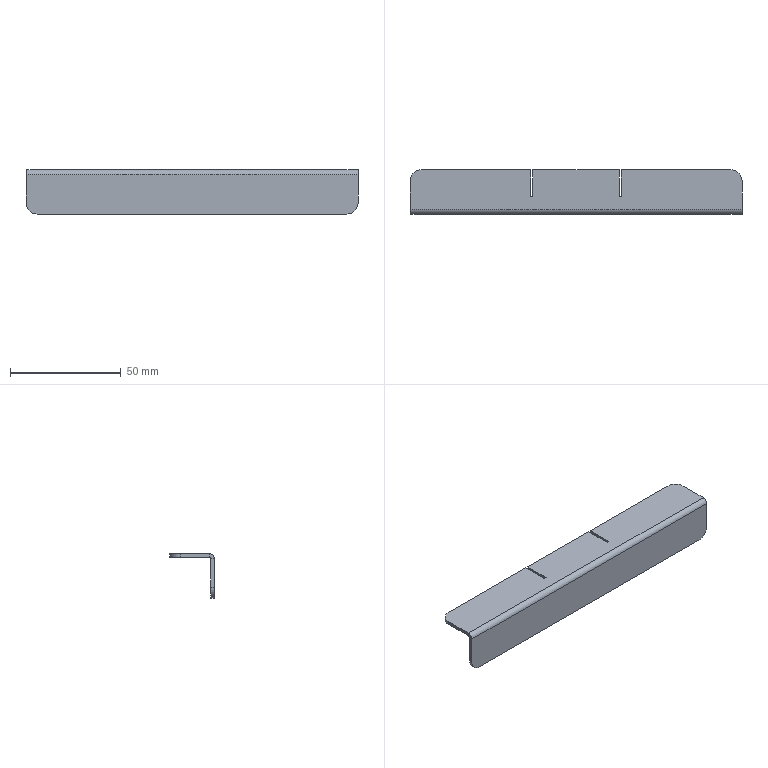Part | SolidWorks | features EdgeFlange 1, Fillet 1, FlatPattern 1, ICE 1, SMBaseFlange 1, SheetMetal 1 | 1 solid | 26 faces | box 150 x 20 x 20 mm | volume 8451 mm3 | plane 20 | cylinder 6 | commonest cylinder face diameters 10 x4 1.473 x1 4.473 x1
STEP:
#1=CARTESIAN_POINT('',(20.5,6.5,10.));
#2=VERTEX_POINT('',#1);
#3=CARTESIAN_POINT('',(19.5,6.5,10.));
#4=VERTEX_POINT('',#3);
#5=CARTESIAN_POINT('',(20.5,6.5,10.));
#6=DIRECTION('',(-1.,0.,0.));
#7=VECTOR('',#6,1000.);
#8=LINE('',#5,#7);
#9=EDGE_CURVE('',#2,#4,#8,.T.);
#10=ORIENTED_EDGE('',*,*,#9,.T.);
#11=CARTESIAN_POINT('',(19.5,18.5,10.));
#12=VERTEX_POINT('',#11);
#13=CARTESIAN_POINT('',(19.5,42.736,10.));
#14=DIRECTION('',(0.,1.,0.));
#15=VECTOR('',#14,1000.);
#16=LINE('',#13,#15);
#17=EDGE_CURVE('',#4,#12,#16,.T.);
#18=ORIENTED_EDGE('',*,*,#17,.T.);
#19=CARTESIAN_POINT('',(-19.5,18.5,10.));
#20=VERTEX_POINT('',#19);
#21=CARTESIAN_POINT('',(75.,18.5,10.));
#22=DIRECTION('',(1.,0.,0.));
#23=VECTOR('',#22,1000.);
#24=LINE('',#21,#23);
#25=EDGE_CURVE('',#20,#12,#24,.T.);
#26=ORIENTED_EDGE('',*,*,#25,.F.);
#27=CARTESIAN_POINT('',(-19.5,6.5,10.));
#28=VERTEX_POINT('',#27);
#29=CARTESIAN_POINT('',(-19.5,42.736,10.));
#30=DIRECTION('',(0.,-1.,0.));
#31=VECTOR('',#30,1000.);
#32=LINE('',#29,#31);
#33=EDGE_CURVE('',#20,#28,#32,.T.);
#34=ORIENTED_EDGE('',*,*,#33,.T.);
#35=CARTESIAN_POINT('',(-20.5,6.5,10.));
#36=VERTEX_POINT('',#35);
#37=CARTESIAN_POINT('',(-20.5,6.5,10.));
#38=DIRECTION('',(-1.,0.,0.));
#39=VECTOR('',#38,1000.);
#40=LINE('',#37,#39);
#41=EDGE_CURVE('',#28,#36,#40,.T.);
#42=ORIENTED_EDGE('',*,*,#41,.T.);
#43=CARTESIAN_POINT('',(-20.5,18.5,10.));
#44=VERTEX_POINT('',#43);
#45=CARTESIAN_POINT('',(-20.5,42.736,10.));
#46=DIRECTION('',(0.,1.,0.));
#47=VECTOR('',#46,1000.);
#48=LINE('',#45,#47);
#49=EDGE_CURVE('',#36,#44,#48,.T.);
#50=ORIENTED_EDGE('',*,*,#49,.T.);
#51=CARTESIAN_POINT('',(-70.,18.5,10.));
#52=VERTEX_POINT('',#51);
#53=CARTESIAN_POINT('',(75.,18.5,10.));
#54=DIRECTION('',(1.,0.,0.));
#55=VECTOR('',#54,1000.);
#56=LINE('',#53,#55);
#57=EDGE_CURVE('',#52,#44,#56,.T.);
#58=ORIENTED_EDGE('',*,*,#57,.F.);
#59=CARTESIAN_POINT('',(-75.,13.5,10.));
#60=VERTEX_POINT('',#59);
#61=CARTESIAN_POINT('',(-70.,13.5,10.));
#62=DIRECTION('',(0.,0.,1.));
#63=DIRECTION('',(0.,-1.,0.));
#64=AXIS2_PLACEMENT_3D('',#61,#62,#63);
#65=CIRCLE('',#64,5.);
#66=EDGE_CURVE('',#52,#60,#65,.T.);
#67=ORIENTED_EDGE('',*,*,#66,.T.);
#68=CARTESIAN_POINT('',(-75.,0.7366,10.));
#69=VERTEX_POINT('',#68);
#70=CARTESIAN_POINT('',(-75.,18.5,10.));
#71=DIRECTION('',(0.,1.,0.));
#72=VECTOR('',#71,1000.);
#73=LINE('',#70,#72);
#74=EDGE_CURVE('',#69,#60,#73,.T.);
#75=ORIENTED_EDGE('',*,*,#74,.F.);
#76=CARTESIAN_POINT('',(75.,0.7366,10.));
#77=VERTEX_POINT('',#76);
#78=CARTESIAN_POINT('',(0.,0.7366,10.));
#79=DIRECTION('',(1.,0.,0.));
#80=VECTOR('',#79,1000.);
#81=LINE('',#78,#80);
#82=EDGE_CURVE('',#69,#77,#81,.T.);
#83=ORIENTED_EDGE('',*,*,#82,.T.);
#84=CARTESIAN_POINT('',(75.,13.5,10.));
#85=VERTEX_POINT('',#84);
#86=CARTESIAN_POINT('',(75.,0.,10.));
#87=DIRECTION('',(0.,-1.,0.));
#88=VECTOR('',#87,1000.);
#89=LINE('',#86,#88);
#90=EDGE_CURVE('',#85,#77,#89,.T.);
#91=ORIENTED_EDGE('',*,*,#90,.F.);
#92=CARTESIAN_POINT('',(70.,18.5,10.));
#93=VERTEX_POINT('',#92);
#94=CARTESIAN_POINT('',(70.,13.5,10.));
#95=DIRECTION('',(0.,0.,1.));
#96=DIRECTION('',(0.,-1.,0.));
#97=AXIS2_PLACEMENT_3D('',#94,#95,#96);
#98=CIRCLE('',#97,5.);
#99=EDGE_CURVE('',#85,#93,#98,.T.);
#100=ORIENTED_EDGE('',*,*,#99,.T.);
#101=CARTESIAN_POINT('',(20.5,18.5,10.));
#102=VERTEX_POINT('',#101);
#103=CARTESIAN_POINT('',(75.,18.5,10.));
#104=DIRECTION('',(1.,0.,0.));
#105=VECTOR('',#104,1000.);
#106=LINE('',#103,#105);
#107=EDGE_CURVE('',#102,#93,#106,.T.);
#108=ORIENTED_EDGE('',*,*,#107,.F.);
#109=CARTESIAN_POINT('',(20.5,42.736,10.));
#110=DIRECTION('',(0.,-1.,0.));
#111=VECTOR('',#110,1000.);
#112=LINE('',#109,#111);
#113=EDGE_CURVE('',#102,#2,#112,.T.);
#114=ORIENTED_EDGE('',*,*,#113,.T.);
#115=EDGE_LOOP('',(#10,#18,#26,#34,#42,#50,#58,#67,#75,#83,#91,#100,#108,#114));
#116=FACE_OUTER_BOUND('',#115,.T.);
#117=CARTESIAN_POINT('',(0.,0.,10.));
#118=DIRECTION('',(0.,0.,1.));
#119=DIRECTION('',(0.,-1.,0.));
#120=AXIS2_PLACEMENT_3D('',#117,#118,#119);
#121=PLANE('',#120);
#122=ADVANCED_FACE('',(#116),#121,.T.);
#123=CARTESIAN_POINT('',(19.5,6.5,8.5));
#124=VERTEX_POINT('',#123);
#125=CARTESIAN_POINT('',(19.5,18.5,8.5));
#126=VERTEX_POINT('',#125);
#127=CARTESIAN_POINT('',(19.5,0.,8.5));
#128=DIRECTION('',(0.,1.,0.));
#129=VECTOR('',#128,1000.);
#130=LINE('',#127,#129);
#131=EDGE_CURVE('',#124,#126,#130,.T.);
#132=ORIENTED_EDGE('',*,*,#131,.F.);
#133=CARTESIAN_POINT('',(20.5,6.5,8.5));
#134=VERTEX_POINT('',#133);
#135=CARTESIAN_POINT('',(0.,6.5,8.5));
#136=DIRECTION('',(-1.,0.,0.));
#137=VECTOR('',#136,1000.);
#138=LINE('',#135,#137);
#139=EDGE_CURVE('',#134,#124,#138,.T.);
#140=ORIENTED_EDGE('',*,*,#139,.F.);
#141=CARTESIAN_POINT('',(20.5,18.5,8.5));
#142=VERTEX_POINT('',#141);
#143=CARTESIAN_POINT('',(20.5,0.,8.5));
#144=DIRECTION('',(0.,-1.,0.));
#145=VECTOR('',#144,1000.);
#146=LINE('',#143,#145);
#147=EDGE_CURVE('',#142,#134,#146,.T.);
#148=ORIENTED_EDGE('',*,*,#147,.F.);
#149=CARTESIAN_POINT('',(70.,18.5,8.5));
#150=VERTEX_POINT('',#149);
#151=CARTESIAN_POINT('',(0.,18.5,8.5));
#152=DIRECTION('',(1.,0.,0.));
#153=VECTOR('',#152,1000.);
#154=LINE('',#151,#153);
#155=EDGE_CURVE('',#142,#150,#154,.T.);
#156=ORIENTED_EDGE('',*,*,#155,.T.);
#157=CARTESIAN_POINT('',(75.,13.5,8.5));
#158=VERTEX_POINT('',#157);
#159=CARTESIAN_POINT('',(70.,13.5,8.5));
#160=DIRECTION('',(0.,0.,-1.));
#161=DIRECTION('',(0.,-1.,0.));
#162=AXIS2_PLACEMENT_3D('',#159,#160,#161);
#163=CIRCLE('',#162,5.);
#164=EDGE_CURVE('',#150,#158,#163,.T.);
#165=ORIENTED_EDGE('',*,*,#164,.T.);
#166=CARTESIAN_POINT('',(75.,0.7366,8.5));
#167=VERTEX_POINT('',#166);
#168=CARTESIAN_POINT('',(75.,0.,8.5));
#169=DIRECTION('',(0.,-1.,0.));
#170=VECTOR('',#169,1000.);
#171=LINE('',#168,#170);
#172=EDGE_CURVE('',#158,#167,#171,.T.);
#173=ORIENTED_EDGE('',*,*,#172,.T.);
#174=CARTESIAN_POINT('',(-75.,0.7366,8.5));
#175=VERTEX_POINT('',#174);
#176=CARTESIAN_POINT('',(-75.,0.7366,8.5));
#177=DIRECTION('',(1.,0.,0.));
#178=VECTOR('',#177,1000.);
#179=LINE('',#176,#178);
#180=EDGE_CURVE('',#175,#167,#179,.T.);
#181=ORIENTED_EDGE('',*,*,#180,.F.);
#182=CARTESIAN_POINT('',(-75.,13.5,8.5));
#183=VERTEX_POINT('',#182);
#184=CARTESIAN_POINT('',(-75.,0.,8.5));
#185=DIRECTION('',(0.,1.,0.));
#186=VECTOR('',#185,1000.);
#187=LINE('',#184,#186);
#188=EDGE_CURVE('',#175,#183,#187,.T.);
#189=ORIENTED_EDGE('',*,*,#188,.T.);
#190=CARTESIAN_POINT('',(-70.,18.5,8.5));
#191=VERTEX_POINT('',#190);
#192=CARTESIAN_POINT('',(-70.,13.5,8.5));
#193=DIRECTION('',(0.,0.,-1.));
#194=DIRECTION('',(0.,-1.,0.));
#195=AXIS2_PLACEMENT_3D('',#192,#193,#194);
#196=CIRCLE('',#195,5.);
#197=EDGE_CURVE('',#183,#191,#196,.T.);
#198=ORIENTED_EDGE('',*,*,#197,.T.);
#199=CARTESIAN_POINT('',(-20.5,18.5,8.5));
#200=VERTEX_POINT('',#199);
#201=CARTESIAN_POINT('',(0.,18.5,8.5));
#202=DIRECTION('',(1.,0.,0.));
#203=VECTOR('',#202,1000.);
#204=LINE('',#201,#203);
#205=EDGE_CURVE('',#191,#200,#204,.T.);
#206=ORIENTED_EDGE('',*,*,#205,.T.);
#207=CARTESIAN_POINT('',(-20.5,6.5,8.5));
#208=VERTEX_POINT('',#207);
#209=CARTESIAN_POINT('',(-20.5,0.,8.5));
#210=DIRECTION('',(0.,1.,0.));
#211=VECTOR('',#210,1000.);
#212=LINE('',#209,#211);
#213=EDGE_CURVE('',#208,#200,#212,.T.);
#214=ORIENTED_EDGE('',*,*,#213,.F.);
#215=CARTESIAN_POINT('',(-19.5,6.5,8.5));
#216=VERTEX_POINT('',#215);
#217=CARTESIAN_POINT('',(0.,6.5,8.5));
#218=DIRECTION('',(-1.,0.,0.));
#219=VECTOR('',#218,1000.);
#220=LINE('',#217,#219);
#221=EDGE_CURVE('',#216,#208,#220,.T.);
#222=ORIENTED_EDGE('',*,*,#221,.F.);
#223=CARTESIAN_POINT('',(-19.5,18.5,8.5));
#224=VERTEX_POINT('',#223);
#225=CARTESIAN_POINT('',(-19.5,0.,8.5));
#226=DIRECTION('',(0.,-1.,0.));
#227=VECTOR('',#226,1000.);
#228=LINE('',#225,#227);
#229=EDGE_CURVE('',#224,#216,#228,.T.);
#230=ORIENTED_EDGE('',*,*,#229,.F.);
#231=CARTESIAN_POINT('',(0.,18.5,8.5));
#232=DIRECTION('',(1.,0.,0.));
#233=VECTOR('',#232,1000.);
#234=LINE('',#231,#233);
#235=EDGE_CURVE('',#224,#126,#234,.T.);
#236=ORIENTED_EDGE('',*,*,#235,.T.);
#237=EDGE_LOOP('',(#132,#140,#148,#156,#165,#173,#181,#189,#198,#206,#214,#222,#230,#236));
#238=FACE_OUTER_BOUND('',#237,.T.);
#239=CARTESIAN_POINT('',(0.,0.,8.5));
#240=DIRECTION('',(0.,0.,1.));
#241=DIRECTION('',(0.,-1.,0.));
#242=AXIS2_PLACEMENT_3D('',#239,#240,#241);
#243=PLANE('',#242);
#244=ADVANCED_FACE('',(#238),#243,.F.);
#245=ORIENTED_EDGE('',*,*,#25,.T.);
#246=CARTESIAN_POINT('',(19.5,18.5,10.));
#247=DIRECTION('',(0.,0.,-1.));
#248=VECTOR('',#247,1000.);
#249=LINE('',#246,#248);
#250=EDGE_CURVE('',#12,#126,#249,.T.);
#251=ORIENTED_EDGE('',*,*,#250,.T.);
#252=ORIENTED_EDGE('',*,*,#235,.F.);
#253=CARTESIAN_POINT('',(-19.5,18.5,10.));
#254=DIRECTION('',(0.,0.,1.));
#255=VECTOR('',#254,1000.);
#256=LINE('',#253,#255);
#257=EDGE_CURVE('',#224,#20,#256,.T.);
#258=ORIENTED_EDGE('',*,*,#257,.T.);
#259=EDGE_LOOP('',(#245,#251,#252,#258));
#260=FACE_OUTER_BOUND('',#259,.T.);
#261=CARTESIAN_POINT('',(75.,18.5,10.));
#262=DIRECTION('',(0.,1.,0.));
#263=DIRECTION('',(0.,0.,1.));
#264=AXIS2_PLACEMENT_3D('',#261,#262,#263);
#265=PLANE('',#264);
#266=ADVANCED_FACE('',(#260),#265,.T.);
#267=ORIENTED_EDGE('',*,*,#155,.F.);
#268=CARTESIAN_POINT('',(20.5,18.5,10.));
#269=DIRECTION('',(0.,0.,1.));
#270=VECTOR('',#269,1000.);
#271=LINE('',#268,#270);
#272=EDGE_CURVE('',#142,#102,#271,.T.);
#273=ORIENTED_EDGE('',*,*,#272,.T.);
#274=ORIENTED_EDGE('',*,*,#107,.T.);
#275=CARTESIAN_POINT('',(70.,18.5,10.));
#276=DIRECTION('',(0.,0.,-1.));
#277=VECTOR('',#276,1000.);
#278=LINE('',#275,#277);
#279=EDGE_CURVE('',#93,#150,#278,.T.);
#280=ORIENTED_EDGE('',*,*,#279,.T.);
#281=EDGE_LOOP('',(#267,#273,#274,#280));
#282=FACE_OUTER_BOUND('',#281,.T.);
#283=CARTESIAN_POINT('',(75.,18.5,10.));
#284=DIRECTION('',(0.,1.,0.));
#285=DIRECTION('',(0.,0.,1.));
#286=AXIS2_PLACEMENT_3D('',#283,#284,#285);
#287=PLANE('',#286);
#288=ADVANCED_FACE('',(#282),#287,.T.);
#289=ORIENTED_EDGE('',*,*,#57,.T.);
#290=CARTESIAN_POINT('',(-20.5,18.5,10.));
#291=DIRECTION('',(0.,0.,-1.));
#292=VECTOR('',#291,1000.);
#293=LINE('',#290,#292);
#294=EDGE_CURVE('',#44,#200,#293,.T.);
#295=ORIENTED_EDGE('',*,*,#294,.T.);
#296=ORIENTED_EDGE('',*,*,#205,.F.);
#297=CARTESIAN_POINT('',(-70.,18.5,10.));
#298=DIRECTION('',(0.,0.,1.));
#299=VECTOR('',#298,1000.);
#300=LINE('',#297,#299);
#301=EDGE_CURVE('',#191,#52,#300,.T.);
#302=ORIENTED_EDGE('',*,*,#301,.T.);
#303=EDGE_LOOP('',(#289,#295,#296,#302));
#304=FACE_OUTER_BOUND('',#303,.T.);
#305=CARTESIAN_POINT('',(75.,18.5,10.));
#306=DIRECTION('',(0.,1.,0.));
#307=DIRECTION('',(0.,0.,1.));
#308=AXIS2_PLACEMENT_3D('',#305,#306,#307);
#309=PLANE('',#308);
#310=ADVANCED_FACE('',(#304),#309,.T.);
#311=CARTESIAN_POINT('',(75.,-1.5,7.763));
#312=VERTEX_POINT('',#311);
#313=CARTESIAN_POINT('',(75.,-1.5,-5.));
#314=VERTEX_POINT('',#313);
#315=CARTESIAN_POINT('',(75.,-1.5,-10.));
#316=DIRECTION('',(0.,0.,-1.));
#317=VECTOR('',#316,1000.);
#318=LINE('',#315,#317);
#319=EDGE_CURVE('',#312,#314,#318,.T.);
#320=ORIENTED_EDGE('',*,*,#319,.T.);
#321=CARTESIAN_POINT('',(75.,0.,-5.));
#322=VERTEX_POINT('',#321);
#323=CARTESIAN_POINT('',(75.,-1.5,-5.));
#324=DIRECTION('',(0.,1.,0.));
#325=VECTOR('',#324,1000.);
#326=LINE('',#323,#325);
#327=EDGE_CURVE('',#314,#322,#326,.T.);
#328=ORIENTED_EDGE('',*,*,#327,.T.);
#329=CARTESIAN_POINT('',(75.,0.,7.763));
#330=VERTEX_POINT('',#329);
#331=CARTESIAN_POINT('',(75.,0.,-10.));
#332=DIRECTION('',(0.,0.,-1.));
#333=VECTOR('',#332,1000.);
#334=LINE('',#331,#333);
#335=EDGE_CURVE('',#330,#322,#334,.T.);
#336=ORIENTED_EDGE('',*,*,#335,.F.);
#337=CARTESIAN_POINT('',(75.,0.,7.763));
#338=DIRECTION('',(0.,-1.,0.));
#339=VECTOR('',#338,1000.);
#340=LINE('',#337,#339);
#341=EDGE_CURVE('',#330,#312,#340,.T.);
#342=ORIENTED_EDGE('',*,*,#341,.T.);
#343=EDGE_LOOP('',(#320,#328,#336,#342));
#344=FACE_OUTER_BOUND('',#343,.T.);
#345=CARTESIAN_POINT('',(75.,-1.5,-10.));
#346=DIRECTION('',(1.,0.,0.));
#347=DIRECTION('',(0.,0.,-1.));
#348=AXIS2_PLACEMENT_3D('',#345,#346,#347);
#349=PLANE('',#348);
#350=ADVANCED_FACE('',(#344),#349,.T.);
#351=CARTESIAN_POINT('',(70.,-1.5,-10.));
#352=VERTEX_POINT('',#351);
#353=CARTESIAN_POINT('',(-70.,-1.5,-10.));
#354=VERTEX_POINT('',#353);
#355=CARTESIAN_POINT('',(-75.,-1.5,-10.));
#356=DIRECTION('',(-1.,0.,0.));
#357=VECTOR('',#356,1000.);
#358=LINE('',#355,#357);
#359=EDGE_CURVE('',#352,#354,#358,.T.);
#360=ORIENTED_EDGE('',*,*,#359,.F.);
#361=CARTESIAN_POINT('',(70.,-1.5,-5.));
#362=DIRECTION('',(0.,-1.,0.));
#363=DIRECTION('',(0.,0.,1.));
#364=AXIS2_PLACEMENT_3D('',#361,#362,#363);
#365=CIRCLE('',#364,5.);
#366=EDGE_CURVE('',#352,#314,#365,.T.);
#367=ORIENTED_EDGE('',*,*,#366,.T.);
#368=ORIENTED_EDGE('',*,*,#319,.F.);
#369=CARTESIAN_POINT('',(-75.,-1.5,7.763));
#370=VERTEX_POINT('',#369);
#371=CARTESIAN_POINT('',(75.,-1.5,7.763));
#372=DIRECTION('',(-1.,0.,0.));
#373=VECTOR('',#372,1000.);
#374=LINE('',#371,#373);
#375=EDGE_CURVE('',#312,#370,#374,.T.);
#376=ORIENTED_EDGE('',*,*,#375,.T.);
#377=CARTESIAN_POINT('',(-75.,-1.5,-5.));
#378=VERTEX_POINT('',#377);
#379=CARTESIAN_POINT('',(-75.,-1.5,-10.));
#380=DIRECTION('',(0.,0.,1.));
#381=VECTOR('',#380,1000.);
#382=LINE('',#379,#381);
#383=EDGE_CURVE('',#378,#370,#382,.T.);
#384=ORIENTED_EDGE('',*,*,#383,.F.);
#385=CARTESIAN_POINT('',(-70.,-1.5,-5.));
#386=DIRECTION('',(0.,-1.,0.));
#387=DIRECTION('',(0.,0.,1.));
#388=AXIS2_PLACEMENT_3D('',#385,#386,#387);
#389=CIRCLE('',#388,5.);
#390=EDGE_CURVE('',#378,#354,#389,.T.);
#391=ORIENTED_EDGE('',*,*,#390,.T.);
#392=EDGE_LOOP('',(#360,#367,#368,#376,#384,#391));
#393=FACE_OUTER_BOUND('',#392,.T.);
#394=CARTESIAN_POINT('',(0.,-1.5,0.));
#395=DIRECTION('',(0.,1.,0.));
#396=DIRECTION('',(0.,0.,1.));
#397=AXIS2_PLACEMENT_3D('',#394,#395,#396);
#398=PLANE('',#397);
#399=ADVANCED_FACE('',(#393),#398,.F.);
#400=ORIENTED_EDGE('',*,*,#335,.T.);
#401=CARTESIAN_POINT('',(70.,0.,-10.));
#402=VERTEX_POINT('',#401);
#403=CARTESIAN_POINT('',(70.,0.,-5.));
#404=DIRECTION('',(0.,1.,0.));
#405=DIRECTION('',(0.,0.,1.));
#406=AXIS2_PLACEMENT_3D('',#403,#404,#405);
#407=CIRCLE('',#406,5.);
#408=EDGE_CURVE('',#322,#402,#407,.T.);
#409=ORIENTED_EDGE('',*,*,#408,.T.);
#410=CARTESIAN_POINT('',(-70.,0.,-10.));
#411=VERTEX_POINT('',#410);
#412=CARTESIAN_POINT('',(-75.,0.,-10.));
#413=DIRECTION('',(-1.,0.,0.));
#414=VECTOR('',#413,1000.);
#415=LINE('',#412,#414);
#416=EDGE_CURVE('',#402,#411,#415,.T.);
#417=ORIENTED_EDGE('',*,*,#416,.T.);
#418=CARTESIAN_POINT('',(-75.,0.,-5.));
#419=VERTEX_POINT('',#418);
#420=CARTESIAN_POINT('',(-70.,0.,-5.));
#421=DIRECTION('',(0.,1.,0.));
#422=DIRECTION('',(0.,0.,1.));
#423=AXIS2_PLACEMENT_3D('',#420,#421,#422);
#424=CIRCLE('',#423,5.);
#425=EDGE_CURVE('',#411,#419,#424,.T.);
#426=ORIENTED_EDGE('',*,*,#425,.T.);
#427=CARTESIAN_POINT('',(-75.,0.,7.763));
#428=VERTEX_POINT('',#427);
#429=CARTESIAN_POINT('',(-75.,0.,-10.));
#430=DIRECTION('',(0.,0.,1.));
#431=VECTOR('',#430,1000.);
#432=LINE('',#429,#431);
#433=EDGE_CURVE('',#419,#428,#432,.T.);
#434=ORIENTED_EDGE('',*,*,#433,.T.);
#435=CARTESIAN_POINT('',(75.,0.,7.763));
#436=DIRECTION('',(-1.,0.,0.));
#437=VECTOR('',#436,1000.);
#438=LINE('',#435,#437);
#439=EDGE_CURVE('',#330,#428,#438,.T.);
#440=ORIENTED_EDGE('',*,*,#439,.F.);
#441=EDGE_LOOP('',(#400,#409,#417,#426,#434,#440));
#442=FACE_OUTER_BOUND('',#441,.T.);
#443=CARTESIAN_POINT('',(0.,0.,0.));
#444=DIRECTION('',(0.,1.,0.));
#445=DIRECTION('',(0.,0.,1.));
#446=AXIS2_PLACEMENT_3D('',#443,#444,#445);
#447=PLANE('',#446);
#448=ADVANCED_FACE('',(#442),#447,.T.);
#449=ORIENTED_EDGE('',*,*,#433,.F.);
#450=CARTESIAN_POINT('',(-75.,-1.5,-5.));
#451=DIRECTION('',(0.,-1.,0.));
#452=VECTOR('',#451,1000.);
#453=LINE('',#450,#452);
#454=EDGE_CURVE('',#419,#378,#453,.T.);
#455=ORIENTED_EDGE('',*,*,#454,.T.);
#456=ORIENTED_EDGE('',*,*,#383,.T.);
#457=CARTESIAN_POINT('',(-75.,0.,7.763));
#458=DIRECTION('',(0.,-1.,0.));
#459=VECTOR('',#458,1000.);
#460=LINE('',#457,#459);
#461=EDGE_CURVE('',#428,#370,#460,.T.);
#462=ORIENTED_EDGE('',*,*,#461,.F.);
#463=EDGE_LOOP('',(#449,#455,#456,#462));
#464=FACE_OUTER_BOUND('',#463,.T.);
#465=CARTESIAN_POINT('',(-75.,-1.5,-10.));
#466=DIRECTION('',(-1.,0.,0.));
#467=DIRECTION('',(0.,0.,1.));
#468=AXIS2_PLACEMENT_3D('',#465,#466,#467);
#469=PLANE('',#468);
#470=ADVANCED_FACE('',(#464),#469,.T.);
#471=ORIENTED_EDGE('',*,*,#416,.F.);
#472=CARTESIAN_POINT('',(70.,-1.5,-10.));
#473=DIRECTION('',(0.,-1.,0.));
#474=VECTOR('',#473,1000.);
#475=LINE('',#472,#474);
#476=EDGE_CURVE('',#402,#352,#475,.T.);
#477=ORIENTED_EDGE('',*,*,#476,.T.);
#478=ORIENTED_EDGE('',*,*,#359,.T.);
#479=CARTESIAN_POINT('',(-70.,-1.5,-10.));
#480=DIRECTION('',(0.,1.,0.));
#481=VECTOR('',#480,1000.);
#482=LINE('',#479,#481);
#483=EDGE_CURVE('',#354,#411,#482,.T.);
#484=ORIENTED_EDGE('',*,*,#483,.T.);
#485=EDGE_LOOP('',(#471,#477,#478,#484));
#486=FACE_OUTER_BOUND('',#485,.T.);
#487=CARTESIAN_POINT('',(-75.,-1.5,-10.));
#488=DIRECTION('',(0.,0.,-1.));
#489=DIRECTION('',(-1.,0.,0.));
#490=AXIS2_PLACEMENT_3D('',#487,#488,#489);
#491=PLANE('',#490);
#492=ADVANCED_FACE('',(#486),#491,.T.);
#493=CARTESIAN_POINT('',(-75.,0.7366,10.));
#494=DIRECTION('',(0.,0.,1.));
#495=VECTOR('',#494,1000.);
#496=LINE('',#493,#495);
#497=EDGE_CURVE('',#175,#69,#496,.T.);
#498=ORIENTED_EDGE('',*,*,#497,.F.);
#499=CARTESIAN_POINT('',(-75.,0.7366,7.763));
#500=DIRECTION('',(-1.,0.,0.));
#501=DIRECTION('',(0.,0.,-1.));
#502=AXIS2_PLACEMENT_3D('',#499,#500,#501);
#503=CIRCLE('',#502,0.7366);
#504=EDGE_CURVE('',#428,#175,#503,.T.);
#505=ORIENTED_EDGE('',*,*,#504,.F.);
#506=ORIENTED_EDGE('',*,*,#461,.T.);
#507=CARTESIAN_POINT('',(-75.,0.7366,7.763));
#508=DIRECTION('',(-1.,0.,0.));
#509=DIRECTION('',(0.,0.,-1.));
#510=AXIS2_PLACEMENT_3D('',#507,#508,#509);
#511=CIRCLE('',#510,2.237);
#512=EDGE_CURVE('',#370,#69,#511,.T.);
#513=ORIENTED_EDGE('',*,*,#512,.T.);
#514=EDGE_LOOP('',(#498,#505,#506,#513));
#515=FACE_OUTER_BOUND('',#514,.T.);
#516=CARTESIAN_POINT('',(-75.,0.7366,7.763));
#517=DIRECTION('',(-1.,0.,0.));
#518=DIRECTION('',(0.,0.,1.));
#519=AXIS2_PLACEMENT_3D('',#516,#517,#518);
#520=PLANE('',#519);
#521=ADVANCED_FACE('',(#515),#520,.T.);
#522=CARTESIAN_POINT('',(75.,0.7366,7.763));
#523=DIRECTION('',(1.,0.,0.));
#524=DIRECTION('',(0.,0.,-1.));
#525=AXIS2_PLACEMENT_3D('',#522,#523,#524);
#526=CIRCLE('',#525,0.7366);
#527=EDGE_CURVE('',#167,#330,#526,.T.);
#528=ORIENTED_EDGE('',*,*,#527,.F.);
#529=CARTESIAN_POINT('',(75.,0.7366,8.5));
#530=DIRECTION('',(0.,0.,1.));
#531=VECTOR('',#530,1000.);
#532=LINE('',#529,#531);
#533=EDGE_CURVE('',#167,#77,#532,.T.);
#534=ORIENTED_EDGE('',*,*,#533,.T.);
#535=CARTESIAN_POINT('',(75.,0.7366,7.763));
#536=DIRECTION('',(1.,0.,0.));
#537=DIRECTION('',(0.,0.,-1.));
#538=AXIS2_PLACEMENT_3D('',#535,#536,#537);
#539=CIRCLE('',#538,2.237);
#540=EDGE_CURVE('',#77,#312,#539,.T.);
#541=ORIENTED_EDGE('',*,*,#540,.T.);
#542=ORIENTED_EDGE('',*,*,#341,.F.);
#543=EDGE_LOOP('',(#528,#534,#541,#542));
#544=FACE_OUTER_BOUND('',#543,.T.);
#545=CARTESIAN_POINT('',(75.,0.7366,7.763));
#546=DIRECTION('',(-1.,0.,0.));
#547=DIRECTION('',(0.,0.,1.));
#548=AXIS2_PLACEMENT_3D('',#545,#546,#547);
#549=PLANE('',#548);
#550=ADVANCED_FACE('',(#544),#549,.F.);
#551=ORIENTED_EDGE('',*,*,#375,.F.);
#552=ORIENTED_EDGE('',*,*,#540,.F.);
#553=ORIENTED_EDGE('',*,*,#82,.F.);
#554=ORIENTED_EDGE('',*,*,#512,.F.);
#555=EDGE_LOOP('',(#551,#552,#553,#554));
#556=FACE_OUTER_BOUND('',#555,.T.);
#557=CARTESIAN_POINT('',(75.,0.7366,7.763));
#558=DIRECTION('',(1.,0.,0.));
#559=DIRECTION('',(0.,0.,1.));
#560=AXIS2_PLACEMENT_3D('',#557,#558,#559);
#561=CYLINDRICAL_SURFACE('',#560,2.237);
#562=ADVANCED_FACE('',(#556),#561,.T.);
#563=ORIENTED_EDGE('',*,*,#439,.T.);
#564=ORIENTED_EDGE('',*,*,#504,.T.);
#565=ORIENTED_EDGE('',*,*,#180,.T.);
#566=ORIENTED_EDGE('',*,*,#527,.T.);
#567=EDGE_LOOP('',(#563,#564,#565,#566));
#568=FACE_OUTER_BOUND('',#567,.T.);
#569=CARTESIAN_POINT('',(75.,0.7366,7.763));
#570=DIRECTION('',(1.,0.,0.));
#571=DIRECTION('',(0.,0.,1.));
#572=AXIS2_PLACEMENT_3D('',#569,#570,#571);
#573=CYLINDRICAL_SURFACE('',#572,0.7366);
#574=ADVANCED_FACE('',(#568),#573,.F.);
#575=ORIENTED_EDGE('',*,*,#172,.F.);
#576=CARTESIAN_POINT('',(75.,13.5,10.));
#577=DIRECTION('',(0.,0.,1.));
#578=VECTOR('',#577,1000.);
#579=LINE('',#576,#578);
#580=EDGE_CURVE('',#158,#85,#579,.T.);
#581=ORIENTED_EDGE('',*,*,#580,.T.);
#582=ORIENTED_EDGE('',*,*,#90,.T.);
#583=ORIENTED_EDGE('',*,*,#533,.F.);
#584=EDGE_LOOP('',(#575,#581,#582,#583));
#585=FACE_OUTER_BOUND('',#584,.T.);
#586=CARTESIAN_POINT('',(75.,0.,10.));
#587=DIRECTION('',(1.,0.,0.));
#588=DIRECTION('',(0.,1.,0.));
#589=AXIS2_PLACEMENT_3D('',#586,#587,#588);
#590=PLANE('',#589);
#591=ADVANCED_FACE('',(#585),#590,.T.);
#592=ORIENTED_EDGE('',*,*,#74,.T.);
#593=CARTESIAN_POINT('',(-75.,13.5,10.));
#594=DIRECTION('',(0.,0.,-1.));
#595=VECTOR('',#594,1000.);
#596=LINE('',#593,#595);
#597=EDGE_CURVE('',#60,#183,#596,.T.);
#598=ORIENTED_EDGE('',*,*,#597,.T.);
#599=ORIENTED_EDGE('',*,*,#188,.F.);
#600=ORIENTED_EDGE('',*,*,#497,.T.);
#601=EDGE_LOOP('',(#592,#598,#599,#600));
#602=FACE_OUTER_BOUND('',#601,.T.);
#603=CARTESIAN_POINT('',(-75.,18.5,10.));
#604=DIRECTION('',(-1.,0.,0.));
#605=DIRECTION('',(0.,0.,1.));
#606=AXIS2_PLACEMENT_3D('',#603,#604,#605);
#607=PLANE('',#606);
#608=ADVANCED_FACE('',(#602),#607,.T.);
#609=ORIENTED_EDGE('',*,*,#99,.F.);
#610=ORIENTED_EDGE('',*,*,#580,.F.);
#611=ORIENTED_EDGE('',*,*,#164,.F.);
#612=ORIENTED_EDGE('',*,*,#279,.F.);
#613=EDGE_LOOP('',(#609,#610,#611,#612));
#614=FACE_OUTER_BOUND('',#613,.T.);
#615=CARTESIAN_POINT('',(70.,13.5,10.));
#616=DIRECTION('',(0.,0.,-1.));
#617=DIRECTION('',(0.,1.,0.));
#618=AXIS2_PLACEMENT_3D('',#615,#616,#617);
#619=CYLINDRICAL_SURFACE('',#618,5.);
#620=ADVANCED_FACE('',(#614),#619,.T.);
#621=ORIENTED_EDGE('',*,*,#366,.F.);
#622=ORIENTED_EDGE('',*,*,#476,.F.);
#623=ORIENTED_EDGE('',*,*,#408,.F.);
#624=ORIENTED_EDGE('',*,*,#327,.F.);
#625=EDGE_LOOP('',(#621,#622,#623,#624));
#626=FACE_OUTER_BOUND('',#625,.T.);
#627=CARTESIAN_POINT('',(70.,-1.5,-5.));
#628=DIRECTION('',(0.,1.,0.));
#629=DIRECTION('',(0.,0.,1.));
#630=AXIS2_PLACEMENT_3D('',#627,#628,#629);
#631=CYLINDRICAL_SURFACE('',#630,5.);
#632=ADVANCED_FACE('',(#626),#631,.T.);
#633=ORIENTED_EDGE('',*,*,#390,.F.);
#634=ORIENTED_EDGE('',*,*,#454,.F.);
#635=ORIENTED_EDGE('',*,*,#425,.F.);
#636=ORIENTED_EDGE('',*,*,#483,.F.);
#637=EDGE_LOOP('',(#633,#634,#635,#636));
#638=FACE_OUTER_BOUND('',#637,.T.);
#639=CARTESIAN_POINT('',(-70.,-1.5,-5.));
#640=DIRECTION('',(0.,1.,0.));
#641=DIRECTION('',(0.,0.,1.));
#642=AXIS2_PLACEMENT_3D('',#639,#640,#641);
#643=CYLINDRICAL_SURFACE('',#642,5.);
#644=ADVANCED_FACE('',(#638),#643,.T.);
#645=ORIENTED_EDGE('',*,*,#66,.F.);
#646=ORIENTED_EDGE('',*,*,#301,.F.);
#647=ORIENTED_EDGE('',*,*,#197,.F.);
#648=ORIENTED_EDGE('',*,*,#597,.F.);
#649=EDGE_LOOP('',(#645,#646,#647,#648));
#650=FACE_OUTER_BOUND('',#649,.T.);
#651=CARTESIAN_POINT('',(-70.,13.5,10.));
#652=DIRECTION('',(0.,0.,-1.));
#653=DIRECTION('',(0.,1.,0.));
#654=AXIS2_PLACEMENT_3D('',#651,#652,#653);
#655=CYLINDRICAL_SURFACE('',#654,5.);
#656=ADVANCED_FACE('',(#650),#655,.T.);
#657=ORIENTED_EDGE('',*,*,#221,.T.);
#658=CARTESIAN_POINT('',(-20.5,6.5,-10.));
#659=DIRECTION('',(0.,0.,1.));
#660=VECTOR('',#659,1000.);
#661=LINE('',#658,#660);
#662=EDGE_CURVE('',#208,#36,#661,.T.);
#663=ORIENTED_EDGE('',*,*,#662,.T.);
#664=ORIENTED_EDGE('',*,*,#41,.F.);
#665=CARTESIAN_POINT('',(-19.5,6.5,-10.));
#666=DIRECTION('',(0.,0.,1.));
#667=VECTOR('',#666,1000.);
#668=LINE('',#665,#667);
#669=EDGE_CURVE('',#216,#28,#668,.T.);
#670=ORIENTED_EDGE('',*,*,#669,.F.);
#671=EDGE_LOOP('',(#657,#663,#664,#670));
#672=FACE_OUTER_BOUND('',#671,.T.);
#673=CARTESIAN_POINT('',(-20.5,6.5,-10.));
#674=DIRECTION('',(0.,1.,0.));
#675=DIRECTION('',(0.,0.,1.));
#676=AXIS2_PLACEMENT_3D('',#673,#674,#675);
#677=PLANE('',#676);
#678=ADVANCED_FACE('',(#672),#677,.T.);
#679=ORIENTED_EDGE('',*,*,#229,.T.);
#680=ORIENTED_EDGE('',*,*,#669,.T.);
#681=ORIENTED_EDGE('',*,*,#33,.F.);
#682=ORIENTED_EDGE('',*,*,#257,.F.);
#683=EDGE_LOOP('',(#679,#680,#681,#682));
#684=FACE_OUTER_BOUND('',#683,.T.);
#685=CARTESIAN_POINT('',(-19.5,42.736,-10.));
#686=DIRECTION('',(-1.,0.,0.));
#687=DIRECTION('',(0.,0.,1.));
#688=AXIS2_PLACEMENT_3D('',#685,#686,#687);
#689=PLANE('',#688);
#690=ADVANCED_FACE('',(#684),#689,.T.);
#691=ORIENTED_EDGE('',*,*,#213,.T.);
#692=ORIENTED_EDGE('',*,*,#294,.F.);
#693=ORIENTED_EDGE('',*,*,#49,.F.);
#694=ORIENTED_EDGE('',*,*,#662,.F.);
#695=EDGE_LOOP('',(#691,#692,#693,#694));
#696=FACE_OUTER_BOUND('',#695,.T.);
#697=CARTESIAN_POINT('',(-20.5,42.736,-10.));
#698=DIRECTION('',(1.,0.,0.));
#699=DIRECTION('',(0.,0.,-1.));
#700=AXIS2_PLACEMENT_3D('',#697,#698,#699);
#701=PLANE('',#700);
#702=ADVANCED_FACE('',(#696),#701,.T.);
#703=ORIENTED_EDGE('',*,*,#139,.T.);
#704=CARTESIAN_POINT('',(19.5,6.5,-10.));
#705=DIRECTION('',(0.,0.,1.));
#706=VECTOR('',#705,1000.);
#707=LINE('',#704,#706);
#708=EDGE_CURVE('',#124,#4,#707,.T.);
#709=ORIENTED_EDGE('',*,*,#708,.T.);
#710=ORIENTED_EDGE('',*,*,#9,.F.);
#711=CARTESIAN_POINT('',(20.5,6.5,-10.));
#712=DIRECTION('',(0.,0.,1.));
#713=VECTOR('',#712,1000.);
#714=LINE('',#711,#713);
#715=EDGE_CURVE('',#134,#2,#714,.T.);
#716=ORIENTED_EDGE('',*,*,#715,.F.);
#717=EDGE_LOOP('',(#703,#709,#710,#716));
#718=FACE_OUTER_BOUND('',#717,.T.);
#719=CARTESIAN_POINT('',(20.5,6.5,-10.));
#720=DIRECTION('',(0.,1.,0.));
#721=DIRECTION('',(0.,0.,1.));
#722=AXIS2_PLACEMENT_3D('',#719,#720,#721);
#723=PLANE('',#722);
#724=ADVANCED_FACE('',(#718),#723,.T.);
#725=ORIENTED_EDGE('',*,*,#131,.T.);
#726=ORIENTED_EDGE('',*,*,#250,.F.);
#727=ORIENTED_EDGE('',*,*,#17,.F.);
#728=ORIENTED_EDGE('',*,*,#708,.F.);
#729=EDGE_LOOP('',(#725,#726,#727,#728));
#730=FACE_OUTER_BOUND('',#729,.T.);
#731=CARTESIAN_POINT('',(19.5,42.736,-10.));
#732=DIRECTION('',(1.,0.,0.));
#733=DIRECTION('',(0.,0.,-1.));
#734=AXIS2_PLACEMENT_3D('',#731,#732,#733);
#735=PLANE('',#734);
#736=ADVANCED_FACE('',(#730),#735,.T.);
#737=ORIENTED_EDGE('',*,*,#147,.T.);
#738=ORIENTED_EDGE('',*,*,#715,.T.);
#739=ORIENTED_EDGE('',*,*,#113,.F.);
#740=ORIENTED_EDGE('',*,*,#272,.F.);
#741=EDGE_LOOP('',(#737,#738,#739,#740));
#742=FACE_OUTER_BOUND('',#741,.T.);
#743=CARTESIAN_POINT('',(20.5,42.736,-10.));
#744=DIRECTION('',(-1.,0.,0.));
#745=DIRECTION('',(0.,0.,1.));
#746=AXIS2_PLACEMENT_3D('',#743,#744,#745);
#747=PLANE('',#746);
#748=ADVANCED_FACE('',(#742),#747,.T.);
#749=CLOSED_SHELL('',(#122,#244,#266,#288,#310,#350,#399,#448,#470,#492,#521,#550,#562,#574,#591,#608,#620,#632,#644,#656,#678,#690,#702,#724,#736,#748));
#750=MANIFOLD_SOLID_BREP('',#749);
#751=CARTESIAN_POINT('',(0.,0.,0.));
#752=DIRECTION('',(0.,0.,1.));
#753=DIRECTION('',(1.,0.,0.));
#754=AXIS2_PLACEMENT_3D('',#751,#752,#753);
#755=(LENGTH_UNIT()NAMED_UNIT(*)SI_UNIT(.MILLI.,.METRE.));
#756=UNCERTAINTY_MEASURE_WITH_UNIT(LENGTH_MEASURE(0.00001),#755,'','');
#757=(NAMED_UNIT(*)PLANE_ANGLE_UNIT()SI_UNIT($,.RADIAN.));
#758=(NAMED_UNIT(*)SI_UNIT($,.STERADIAN.)SOLID_ANGLE_UNIT());
#759=(GEOMETRIC_REPRESENTATION_CONTEXT(3)GLOBAL_UNCERTAINTY_ASSIGNED_CONTEXT((#756))GLOBAL_UNIT_ASSIGNED_CONTEXT((#755,#757,#758))REPRESENTATION_CONTEXT('',''));
#760=ADVANCED_BREP_SHAPE_REPRESENTATION('',(#750,#754),#759);